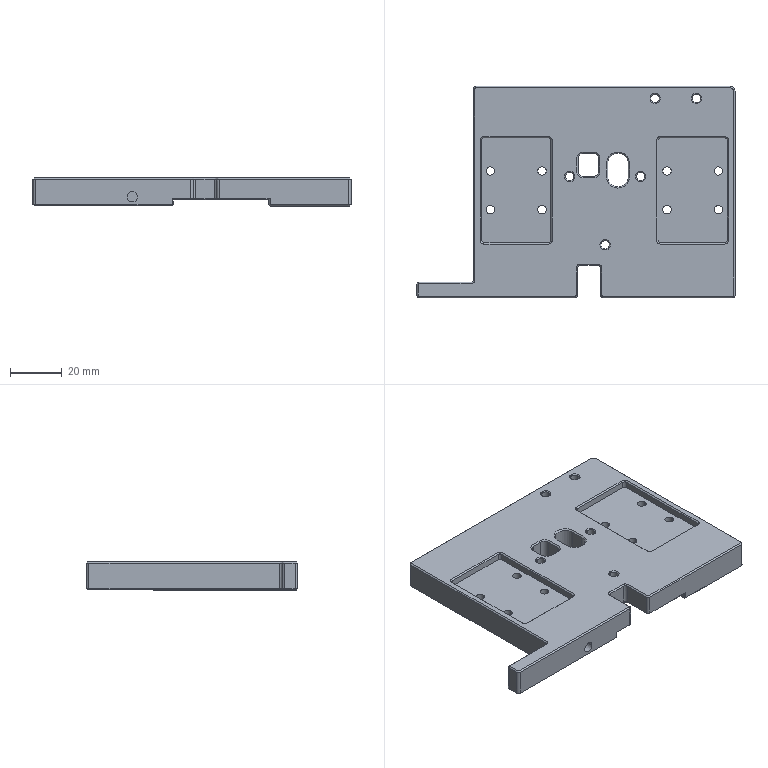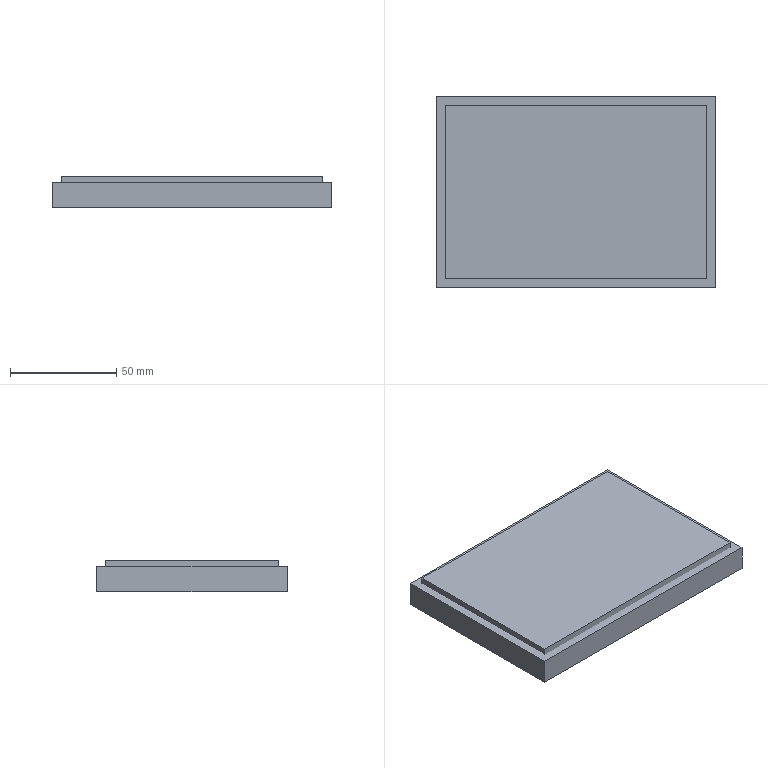CAM job | NX | 3-axis milling, drilling | part box 123.41 x 82 x 11.078 mm | stock box 131.41 x 90.001 x 15.079 mm
Tools:
number,name,description,diameter,corner_radius,flute_length,length,flutes
1,D63,Milling Tool-5 Parameters,63.0,0.0,50.0,75.0,2
2,D4A45,Milling Tool-5 Parameters,4.0,0.0,2.0,2.0,2
13,3.3ZT,Drilling Tool,3.3,0.0,35.0,50.0,2
10,D10,Milling Tool-5 Parameters,10.0,0.0,50.0,75.0,2
6,D6,Milling Tool-5 Parameters,6.0,0.0,50.0,75.0,2
4,D4,Milling Tool-5 Parameters,4.0,0.0,50.0,75.0,2
12,D2,Milling Tool-5 Parameters,2.0,0.0,50.0,75.0,2
Operations:
program,operation,operation_type,tool,method,geometry_group,spindle_rpm,surface_speed,feed_per_tooth,feed_cut,feed_plunge,cut_length_mm,path_length_mm,cut_time_min,machine_time_min
1虎钳,FLOOR_WALL,VolumeBased25DMillingOperation,D63,METHOD,A,6500.0,1286.0,0.0962,1250.0,100.0,660.028,714.028,0.528,0.5334
1虎钳,DRILLING_COPY,Operation,D4A45,METHOD,A,5000.0,62.0,0.025,250.0,0.0,52.0,433.829,0.208,0.2462
1虎钳,DRILLING_COPY_COPY_COPY_COPY_COPY_COPY,Operation,3.3ZT,METHOD,A,1910.0,21.0,0.0471,180.0,0.0,201.388,732.606,1.119,1.172
1虎钳,ADAPTIVE_MILLING,CavityMilling,D10,METHOD,A,9500.0,298.0,0.1579,3000.0,1000.0,9118.432,9407.292,3.485,3.514
1虎钳,CAVITY_MILL_COPY,CavityMilling,D6,METHOD,A,9500.0,119.0,0.1053,2000.0,1000.0,1297.621,2469.995,0.7452,0.8624
1虎钳,ZLEVEL_PROFILE_COPY_COPY_1_COPY,ZLevelMilling,D6,METHOD,A,9500.0,179.0,0.1158,2200.0,1000.0,541.399,684.324,0.2873,0.3016
1虎钳,CAVITY_MILL_COPY_COPY,CavityMilling,D4,METHOD,A,9500.0,119.0,0.1053,2000.0,1000.0,1173.223,2855.81,0.7476,0.9158
1虎钳,ZLEVEL_PROFILE_COPY_COPY_COPY_COPY,ZLevelMilling,D4,MILL_FINISH,A,9500.0,119.0,0.0632,1200.0,1000.0,446.622,525.777,0.3725,0.3805
1虎钳,ZLEVEL_PROFILE_COPY_COPY_COPY_COPY_COPY,ZLevelMilling,D4,MILL_FINISH,A,9500.0,119.0,0.0632,1200.0,1000.0,49.242,206.092,0.0418,0.0575
1虎钳,FLOOR_WALL_1,VolumeBased25DMillingOperation,D4,METHOD,A,9500.0,119.0,0.0526,1000.0,100.0,1241.741,1426.252,1.242,1.26
1虎钳,CAVITY_MILL_COPY_COPY_COPY,CavityMilling,D2,METHOD,A,9500.0,59.0,0.0526,1000.0,1000.0,1582.908,3369.503,1.583,1.762
1虎钳,ZLEVEL_PROFILE_1_COPY_1_COPY_COPY,ZLevelMilling,D4A45,METHOD,A,9500.0,179.0,0.0526,1000.0,100.0,830.252,1841.945,0.8303,0.9314
2,ZLEVEL_PROFILE_COPY_COPY_COPY_COPY_COPY_1,ZLevelMilling,D10,MILL_FINISH,B,9500.0,119.0,0.0632,1200.0,1000.0,681.011,956.131,0.57,0.5976
2,FLOOR_WALL_COPY,VolumeBased25DMillingOperation,D63,METHOD,B,6500.0,1286.0,0.0962,1250.0,100.0,2512.112,3317.967,2.01,2.09
2,CAVITY_MILL_COPY_COPY_1,CavityMilling,D10,METHOD,B,9500.0,298.0,0.1053,2000.0,1000.0,2628.974,2945.042,1.489,1.52
2,CAVITY_MILL_COPY_COPY_COPY_1,CavityMilling,D4,METHOD,B,9500.0,119.0,0.1053,2000.0,1000.0,40.534,118.047,0.0237,0.0315
2,FLOOR_WALL_1_COPY,VolumeBased25DMillingOperation,D4,METHOD,B,9500.0,119.0,0.0526,1000.0,100.0,2584.023,2886.059,2.584,2.614
2,FLOOR_WALL_1_COPY_COPY,VolumeBased25DMillingOperation,D4,METHOD,B,9500.0,119.0,0.0526,1000.0,100.0,1701.62,1934.583,1.702,1.725
2,HOLE_MILLING,CylinderMilling,D4,METHOD,B,9500.0,179.0,0.0789,1500.0,100.0,889.38,1582.833,0.5929,0.6623
2,ZLEVEL_PROFILE_1_COPY_1_COPY_COPY_COPY,ZLevelMilling,D4A45,METHOD,B,9500.0,179.0,0.0526,1000.0,100.0,611.23,1554.201,0.6112,0.7055
2,ZLEVEL_PROFILE_1_COPY_1_COPY_COPY_COPY_COPY,ZLevelMilling,D4A45,METHOD,B,9500.0,179.0,0.0526,1000.0,100.0,222.053,875.664,0.2221,0.2874
2,ZLEVEL_PROFILE_1_COPY_1_COPY_COPY_COPY_COPY_COPY,ZLevelMilling,D4A45,METHOD,B,9500.0,179.0,0.0526,1000.0,100.0,82.052,326.475,0.0821,0.1065
2,刀补4,VolumeBased25DMillingOperation,D4,METHOD,B,9500.0,119.0,0.0526,1000.0,100.0,150.645,304.357,0.1506,0.166